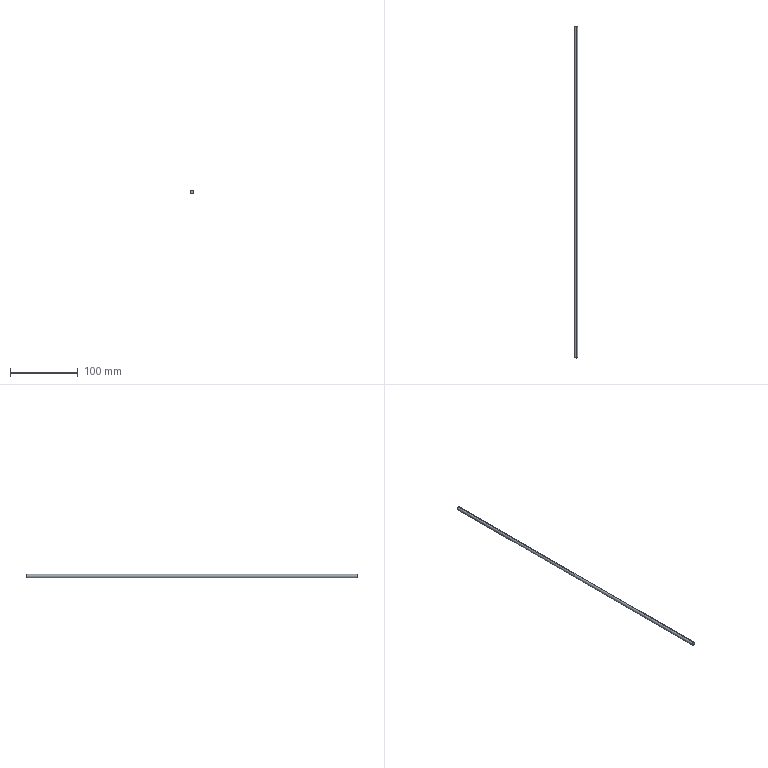Part | STEP file | Cleaning nozzle shaft | 1 solid | 4 faces | box 5 x 490 x 5 mm | volume 9621 mm3 | cylinder 2 | plane 2 | commonest cylinder face diameters 5 x2
STEP:
#1=CARTESIAN_POINT('',(0.,0.,0.));
#2=DIRECTION('',(0.,0.,1.));
#3=DIRECTION('',(1.,0.,0.));
#4=AXIS2_PLACEMENT_3D('',#1,#2,#3);
#5=CARTESIAN_POINT('',(0.,490.,2.5));
#6=VERTEX_POINT('',#5);
#7=CARTESIAN_POINT('',(0.,490.,-2.5));
#8=VERTEX_POINT('',#7);
#9=CARTESIAN_POINT('',(0.,490.,0.));
#10=DIRECTION('',(0.,1.,0.));
#11=DIRECTION('',(0.,0.,1.));
#12=AXIS2_PLACEMENT_3D('',#9,#10,#11);
#13=CIRCLE('',#12,2.5);
#14=CARTESIAN_POINT('',(0.,490.,0.));
#15=DIRECTION('',(0.,-1.,0.));
#16=DIRECTION('',(0.,0.,-1.));
#17=AXIS2_PLACEMENT_3D('',#14,#15,#16);
#18=CYLINDRICAL_SURFACE('',#17,2.5);
#19=CARTESIAN_POINT('',(3.142,0.));
#20=DIRECTION('',(-1.,0.));
#21=VECTOR('',#20,1.);
#22=LINE('',#19,#21);
#23=(GEOMETRIC_REPRESENTATION_CONTEXT(2)PARAMETRIC_REPRESENTATION_CONTEXT()REPRESENTATION_CONTEXT('',''));
#24=DEFINITIONAL_REPRESENTATION('',(#22),#23);
#25=PCURVE('',#18,#24);
#26=CARTESIAN_POINT('',(0.,490.,0.));
#27=DIRECTION('',(0.,1.,0.));
#28=DIRECTION('',(0.,0.,1.));
#29=AXIS2_PLACEMENT_3D('',#26,#27,#28);
#30=PLANE('',#29);
#31=CARTESIAN_POINT('',(0.,0.));
#32=DIRECTION('',(1.,0.));
#33=AXIS2_PLACEMENT_2D('',#31,#32);
#34=CIRCLE('',#33,2.5);
#35=(GEOMETRIC_REPRESENTATION_CONTEXT(2)PARAMETRIC_REPRESENTATION_CONTEXT()REPRESENTATION_CONTEXT('',''));
#36=DEFINITIONAL_REPRESENTATION('',(#34),#35);
#37=PCURVE('',#30,#36);
#38=SURFACE_CURVE('',#13,(#25,#37),.PCURVE_S1.);
#39=EDGE_CURVE('',#6,#8,#38,.T.);
#40=ORIENTED_EDGE('',*,*,#39,.F.);
#41=CARTESIAN_POINT('',(0.,0.,2.5));
#42=VERTEX_POINT('',#41);
#43=CARTESIAN_POINT('',(0.,490.,2.5));
#44=DIRECTION('',(0.,-1.,0.));
#45=VECTOR('',#44,1.);
#46=LINE('',#43,#45);
#47=CARTESIAN_POINT('',(3.142,0.));
#48=DIRECTION('',(0.,1.));
#49=VECTOR('',#48,1.);
#50=LINE('',#47,#49);
#51=(GEOMETRIC_REPRESENTATION_CONTEXT(2)PARAMETRIC_REPRESENTATION_CONTEXT()REPRESENTATION_CONTEXT('',''));
#52=DEFINITIONAL_REPRESENTATION('',(#50),#51);
#53=PCURVE('',#18,#52);
#54=CARTESIAN_POINT('',(0.,490.,0.));
#55=DIRECTION('',(0.,-1.,0.));
#56=DIRECTION('',(0.,0.,-1.));
#57=AXIS2_PLACEMENT_3D('',#54,#55,#56);
#58=CYLINDRICAL_SURFACE('',#57,2.5);
#59=CARTESIAN_POINT('',(3.142,0.));
#60=DIRECTION('',(0.,1.));
#61=VECTOR('',#60,1.);
#62=LINE('',#59,#61);
#63=(GEOMETRIC_REPRESENTATION_CONTEXT(2)PARAMETRIC_REPRESENTATION_CONTEXT()REPRESENTATION_CONTEXT('',''));
#64=DEFINITIONAL_REPRESENTATION('',(#62),#63);
#65=PCURVE('',#58,#64);
#66=SURFACE_CURVE('',#46,(#53,#65),.PCURVE_S1.);
#67=EDGE_CURVE('',#6,#42,#66,.T.);
#68=ORIENTED_EDGE('',*,*,#67,.T.);
#69=CARTESIAN_POINT('',(0.,0.,-2.5));
#70=VERTEX_POINT('',#69);
#71=CARTESIAN_POINT('',(0.,0.,0.));
#72=DIRECTION('',(0.,1.,0.));
#73=DIRECTION('',(0.,0.,1.));
#74=AXIS2_PLACEMENT_3D('',#71,#72,#73);
#75=CIRCLE('',#74,2.5);
#76=CARTESIAN_POINT('',(3.142,490.));
#77=DIRECTION('',(-1.,0.));
#78=VECTOR('',#77,1.);
#79=LINE('',#76,#78);
#80=(GEOMETRIC_REPRESENTATION_CONTEXT(2)PARAMETRIC_REPRESENTATION_CONTEXT()REPRESENTATION_CONTEXT('',''));
#81=DEFINITIONAL_REPRESENTATION('',(#79),#80);
#82=PCURVE('',#18,#81);
#83=CARTESIAN_POINT('',(0.,0.,0.));
#84=DIRECTION('',(0.,1.,0.));
#85=DIRECTION('',(0.,0.,1.));
#86=AXIS2_PLACEMENT_3D('',#83,#84,#85);
#87=PLANE('',#86);
#88=CARTESIAN_POINT('',(0.,0.));
#89=DIRECTION('',(1.,0.));
#90=AXIS2_PLACEMENT_2D('',#88,#89);
#91=CIRCLE('',#90,2.5);
#92=(GEOMETRIC_REPRESENTATION_CONTEXT(2)PARAMETRIC_REPRESENTATION_CONTEXT()REPRESENTATION_CONTEXT('',''));
#93=DEFINITIONAL_REPRESENTATION('',(#91),#92);
#94=PCURVE('',#87,#93);
#95=SURFACE_CURVE('',#75,(#82,#94),.PCURVE_S1.);
#96=EDGE_CURVE('',#42,#70,#95,.T.);
#97=ORIENTED_EDGE('',*,*,#96,.T.);
#98=CARTESIAN_POINT('',(0.,490.,-2.5));
#99=DIRECTION('',(0.,-1.,0.));
#100=VECTOR('',#99,1.);
#101=LINE('',#98,#100);
#102=CARTESIAN_POINT('',(0.,0.));
#103=DIRECTION('',(0.,1.));
#104=VECTOR('',#103,1.);
#105=LINE('',#102,#104);
#106=(GEOMETRIC_REPRESENTATION_CONTEXT(2)PARAMETRIC_REPRESENTATION_CONTEXT()REPRESENTATION_CONTEXT('',''));
#107=DEFINITIONAL_REPRESENTATION('',(#105),#106);
#108=PCURVE('',#18,#107);
#109=CARTESIAN_POINT('',(6.283,0.));
#110=DIRECTION('',(0.,1.));
#111=VECTOR('',#110,1.);
#112=LINE('',#109,#111);
#113=(GEOMETRIC_REPRESENTATION_CONTEXT(2)PARAMETRIC_REPRESENTATION_CONTEXT()REPRESENTATION_CONTEXT('',''));
#114=DEFINITIONAL_REPRESENTATION('',(#112),#113);
#115=PCURVE('',#58,#114);
#116=SURFACE_CURVE('',#101,(#108,#115),.PCURVE_S1.);
#117=EDGE_CURVE('',#8,#70,#116,.T.);
#118=ORIENTED_EDGE('',*,*,#117,.F.);
#119=EDGE_LOOP('',(#40,#68,#97,#118));
#120=FACE_BOUND('',#119,.T.);
#121=ADVANCED_FACE('',(#120),#18,.T.);
#122=ORIENTED_EDGE('',*,*,#67,.F.);
#123=CARTESIAN_POINT('',(0.,490.,0.));
#124=DIRECTION('',(0.,1.,0.));
#125=DIRECTION('',(0.,0.,1.));
#126=AXIS2_PLACEMENT_3D('',#123,#124,#125);
#127=CIRCLE('',#126,2.5);
#128=CARTESIAN_POINT('',(9.425,0.));
#129=DIRECTION('',(-1.,0.));
#130=VECTOR('',#129,1.);
#131=LINE('',#128,#130);
#132=(GEOMETRIC_REPRESENTATION_CONTEXT(2)PARAMETRIC_REPRESENTATION_CONTEXT()REPRESENTATION_CONTEXT('',''));
#133=DEFINITIONAL_REPRESENTATION('',(#131),#132);
#134=PCURVE('',#58,#133);
#135=CARTESIAN_POINT('',(0.,0.));
#136=DIRECTION('',(1.,0.));
#137=AXIS2_PLACEMENT_2D('',#135,#136);
#138=CIRCLE('',#137,2.5);
#139=(GEOMETRIC_REPRESENTATION_CONTEXT(2)PARAMETRIC_REPRESENTATION_CONTEXT()REPRESENTATION_CONTEXT('',''));
#140=DEFINITIONAL_REPRESENTATION('',(#138),#139);
#141=PCURVE('',#30,#140);
#142=SURFACE_CURVE('',#127,(#134,#141),.PCURVE_S1.);
#143=EDGE_CURVE('',#8,#6,#142,.T.);
#144=ORIENTED_EDGE('',*,*,#143,.F.);
#145=ORIENTED_EDGE('',*,*,#117,.T.);
#146=CARTESIAN_POINT('',(0.,0.,0.));
#147=DIRECTION('',(0.,1.,0.));
#148=DIRECTION('',(0.,0.,1.));
#149=AXIS2_PLACEMENT_3D('',#146,#147,#148);
#150=CIRCLE('',#149,2.5);
#151=CARTESIAN_POINT('',(9.425,490.));
#152=DIRECTION('',(-1.,0.));
#153=VECTOR('',#152,1.);
#154=LINE('',#151,#153);
#155=(GEOMETRIC_REPRESENTATION_CONTEXT(2)PARAMETRIC_REPRESENTATION_CONTEXT()REPRESENTATION_CONTEXT('',''));
#156=DEFINITIONAL_REPRESENTATION('',(#154),#155);
#157=PCURVE('',#58,#156);
#158=CARTESIAN_POINT('',(0.,0.));
#159=DIRECTION('',(1.,0.));
#160=AXIS2_PLACEMENT_2D('',#158,#159);
#161=CIRCLE('',#160,2.5);
#162=(GEOMETRIC_REPRESENTATION_CONTEXT(2)PARAMETRIC_REPRESENTATION_CONTEXT()REPRESENTATION_CONTEXT('',''));
#163=DEFINITIONAL_REPRESENTATION('',(#161),#162);
#164=PCURVE('',#87,#163);
#165=SURFACE_CURVE('',#150,(#157,#164),.PCURVE_S1.);
#166=EDGE_CURVE('',#70,#42,#165,.T.);
#167=ORIENTED_EDGE('',*,*,#166,.T.);
#168=EDGE_LOOP('',(#122,#144,#145,#167));
#169=FACE_BOUND('',#168,.T.);
#170=ADVANCED_FACE('',(#169),#58,.T.);
#171=ORIENTED_EDGE('',*,*,#143,.T.);
#172=ORIENTED_EDGE('',*,*,#39,.T.);
#173=EDGE_LOOP('',(#171,#172));
#174=FACE_BOUND('',#173,.T.);
#175=ADVANCED_FACE('',(#174),#30,.T.);
#176=ORIENTED_EDGE('',*,*,#166,.F.);
#177=ORIENTED_EDGE('',*,*,#96,.F.);
#178=EDGE_LOOP('',(#176,#177));
#179=FACE_BOUND('',#178,.T.);
#180=ADVANCED_FACE('',(#179),#87,.F.);
#181=CLOSED_SHELL('',(#121,#170,#175,#180));
#182=MANIFOLD_SOLID_BREP('',#181);
#183=(LENGTH_UNIT()NAMED_UNIT(*)SI_UNIT(.MILLI.,.METRE.));
#184=UNCERTAINTY_MEASURE_WITH_UNIT(LENGTH_MEASURE(0.0000001),#183,'','');
#185=(NAMED_UNIT(*)PLANE_ANGLE_UNIT()SI_UNIT($,.RADIAN.));
#186=(NAMED_UNIT(*)SI_UNIT($,.STERADIAN.)SOLID_ANGLE_UNIT());
#187=(GEOMETRIC_REPRESENTATION_CONTEXT(3)GLOBAL_UNCERTAINTY_ASSIGNED_CONTEXT((#184))GLOBAL_UNIT_ASSIGNED_CONTEXT((#183,#185,#186))REPRESENTATION_CONTEXT('',''));
#188=ADVANCED_BREP_SHAPE_REPRESENTATION('',(#4,#182),#187);